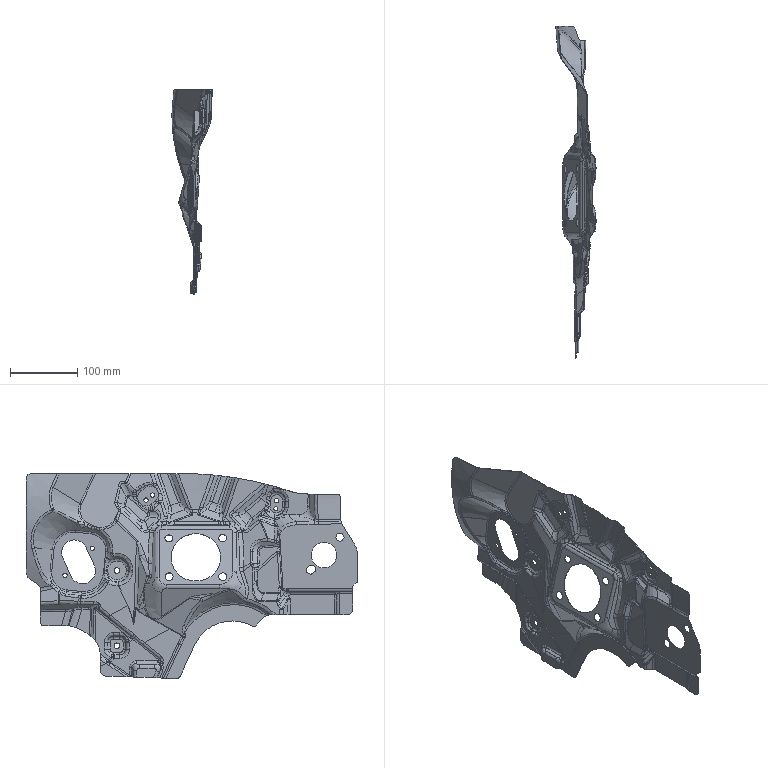Part | 1 solid | 1351 faces | box 60.057 x 494.1 x 305.295 mm | volume 90110 mm3 | spline 899 | cylinder 277 | plane 108 | sphere 36 | other 29 | torus 2 | commonest cylinder face diameters 10 x79 8.4 x39 11.6 x38 16 x21 12 x14 14.4 x12